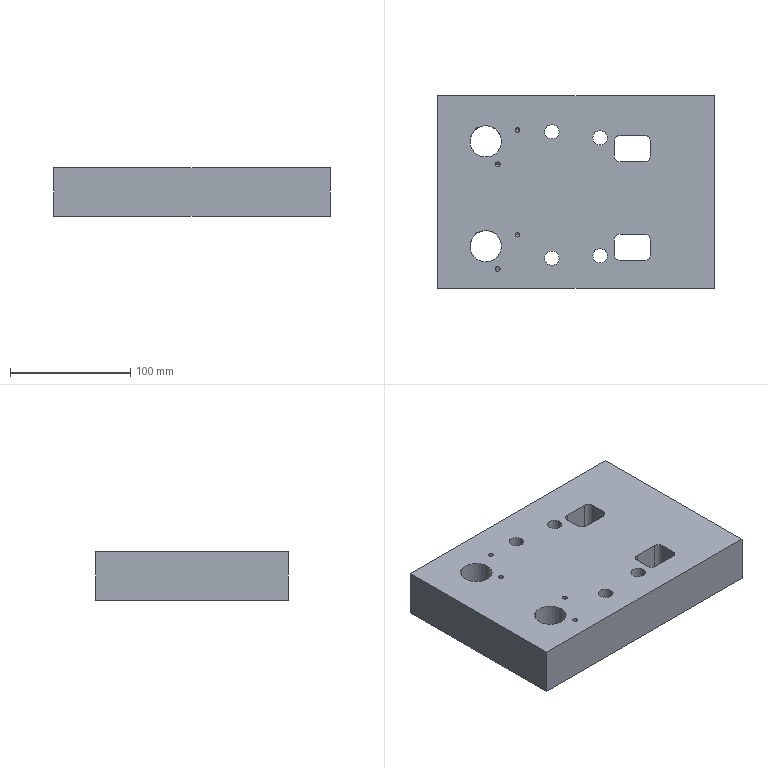Part | 1 solid | 62 faces | box 230 x 160 x 40 mm | volume 1274688 mm3 | cylinder 33 | plane 19 | cone 10 | commonest cylinder face diameters 12 x11 4 x10 10 x8 26 x4